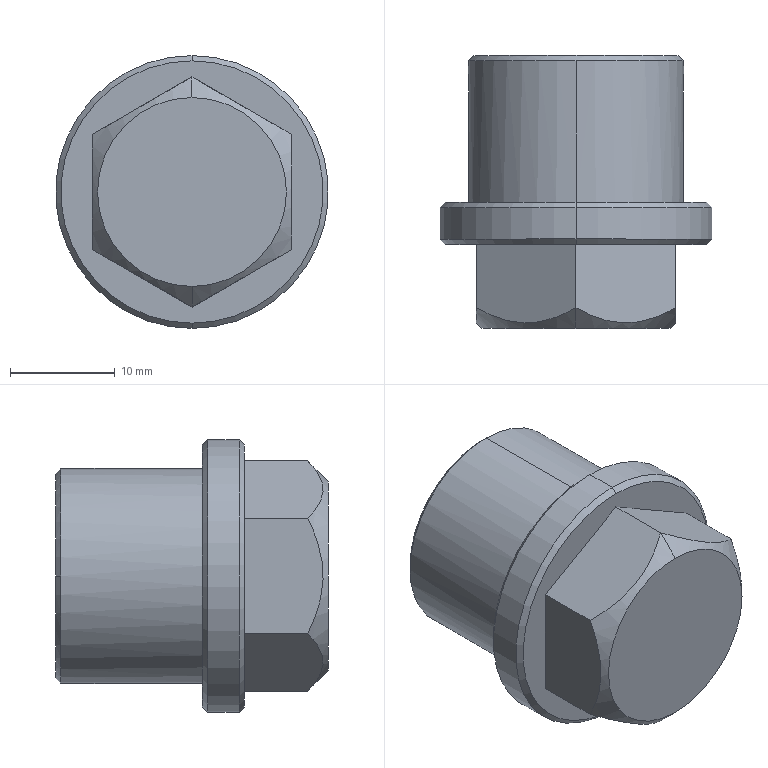Part | STEP file | VD-151208000366A_DN15_X2_76F490 | 1 solid | 22 faces | box 26 x 26 x 26 mm | volume 9182 mm3 | plane 10 | cone 8 | cylinder 4 | commonest cylinder face diameters 20.5 x2 26 x2
STEP:
#1=CARTESIAN_POINT('',(9.75,26.,0.));
#2=VERTEX_POINT('',#1);
#3=CARTESIAN_POINT('',(-9.75,26.,0.));
#4=VERTEX_POINT('',#3);
#5=CARTESIAN_POINT('',(0.,26.,0.));
#6=DIRECTION('',(0.,1.,0.));
#7=DIRECTION('',(1.,0.,0.));
#8=AXIS2_PLACEMENT_3D('',#5,#6,#7);
#9=CIRCLE('',#8,9.75);
#10=EDGE_CURVE('',#2,#4,#9,.T.);
#11=ORIENTED_EDGE('',*,*,#10,.T.);
#12=CARTESIAN_POINT('',(0.,26.,0.));
#13=DIRECTION('',(0.,1.,0.));
#14=DIRECTION('',(-1.,0.,0.));
#15=AXIS2_PLACEMENT_3D('',#12,#13,#14);
#16=CIRCLE('',#15,9.75);
#17=EDGE_CURVE('',#4,#2,#16,.T.);
#18=ORIENTED_EDGE('',*,*,#17,.T.);
#19=EDGE_LOOP('',(#11,#18));
#20=FACE_OUTER_BOUND('',#19,.T.);
#21=CARTESIAN_POINT('',(0.,26.,0.));
#22=DIRECTION('',(0.,1.,0.));
#23=DIRECTION('',(1.,0.,0.));
#24=AXIS2_PLACEMENT_3D('',#21,#22,#23);
#25=PLANE('',#24);
#26=ADVANCED_FACE('',(#20),#25,.T.);
#27=CARTESIAN_POINT('',(-10.25,25.5,0.));
#28=VERTEX_POINT('',#27);
#29=CARTESIAN_POINT('',(-10.25,25.5,0.));
#30=DIRECTION('',(0.7071,0.7071,0.));
#31=VECTOR('',#30,1000.);
#32=LINE('',#29,#31);
#33=EDGE_CURVE('',#28,#4,#32,.T.);
#34=ORIENTED_EDGE('',*,*,#33,.F.);
#35=CARTESIAN_POINT('',(0.,25.5,10.25));
#36=VERTEX_POINT('',#35);
#37=CARTESIAN_POINT('',(0.,25.5,0.));
#38=DIRECTION('',(0.,1.,0.));
#39=DIRECTION('',(-1.,0.,0.));
#40=AXIS2_PLACEMENT_3D('',#37,#38,#39);
#41=CIRCLE('',#40,10.25);
#42=EDGE_CURVE('',#28,#36,#41,.T.);
#43=ORIENTED_EDGE('',*,*,#42,.T.);
#44=CARTESIAN_POINT('',(10.25,25.5,0.));
#45=VERTEX_POINT('',#44);
#46=CARTESIAN_POINT('',(0.,25.5,0.));
#47=DIRECTION('',(0.,1.,0.));
#48=DIRECTION('',(0.,0.,1.));
#49=AXIS2_PLACEMENT_3D('',#46,#47,#48);
#50=CIRCLE('',#49,10.25);
#51=EDGE_CURVE('',#36,#45,#50,.T.);
#52=ORIENTED_EDGE('',*,*,#51,.T.);
#53=CARTESIAN_POINT('',(10.25,25.5,0.));
#54=DIRECTION('',(-0.7071,0.7071,0.));
#55=VECTOR('',#54,1000.);
#56=LINE('',#53,#55);
#57=EDGE_CURVE('',#45,#2,#56,.T.);
#58=ORIENTED_EDGE('',*,*,#57,.T.);
#59=ORIENTED_EDGE('',*,*,#17,.F.);
#60=EDGE_LOOP('',(#34,#43,#52,#58,#59));
#61=FACE_OUTER_BOUND('',#60,.T.);
#62=CARTESIAN_POINT('',(0.,25.75,0.));
#63=DIRECTION('',(0.,-1.,0.));
#64=DIRECTION('',(1.,0.,0.));
#65=AXIS2_PLACEMENT_3D('',#62,#63,#64);
#66=CONICAL_SURFACE('',#65,10.,0.7854);
#67=ADVANCED_FACE('',(#61),#66,.T.);
#68=ORIENTED_EDGE('',*,*,#10,.F.);
#69=ORIENTED_EDGE('',*,*,#57,.F.);
#70=CARTESIAN_POINT('',(0.,25.5,-10.25));
#71=VERTEX_POINT('',#70);
#72=CARTESIAN_POINT('',(0.,25.5,0.));
#73=DIRECTION('',(0.,1.,0.));
#74=DIRECTION('',(1.,0.,0.));
#75=AXIS2_PLACEMENT_3D('',#72,#73,#74);
#76=CIRCLE('',#75,10.25);
#77=EDGE_CURVE('',#45,#71,#76,.T.);
#78=ORIENTED_EDGE('',*,*,#77,.T.);
#79=CARTESIAN_POINT('',(0.,25.5,0.));
#80=DIRECTION('',(0.,1.,0.));
#81=DIRECTION('',(0.,0.,-1.));
#82=AXIS2_PLACEMENT_3D('',#79,#80,#81);
#83=CIRCLE('',#82,10.25);
#84=EDGE_CURVE('',#71,#28,#83,.T.);
#85=ORIENTED_EDGE('',*,*,#84,.T.);
#86=ORIENTED_EDGE('',*,*,#33,.T.);
#87=EDGE_LOOP('',(#68,#69,#78,#85,#86));
#88=FACE_OUTER_BOUND('',#87,.T.);
#89=CARTESIAN_POINT('',(0.,25.75,0.));
#90=DIRECTION('',(0.,-1.,0.));
#91=DIRECTION('',(1.,0.,0.));
#92=AXIS2_PLACEMENT_3D('',#89,#90,#91);
#93=CONICAL_SURFACE('',#92,10.,0.7854);
#94=ADVANCED_FACE('',(#88),#93,.T.);
#95=CARTESIAN_POINT('',(0.,12.,10.25));
#96=VERTEX_POINT('',#95);
#97=CARTESIAN_POINT('',(0.,12.,-10.25));
#98=VERTEX_POINT('',#97);
#99=CARTESIAN_POINT('',(0.,12.,0.));
#100=DIRECTION('',(0.,-1.,0.));
#101=DIRECTION('',(0.,0.,1.));
#102=AXIS2_PLACEMENT_3D('',#99,#100,#101);
#103=CIRCLE('',#102,10.25);
#104=EDGE_CURVE('',#96,#98,#103,.T.);
#105=ORIENTED_EDGE('',*,*,#104,.F.);
#106=CARTESIAN_POINT('',(0.,25.5,10.25));
#107=DIRECTION('',(0.,-1.,0.));
#108=VECTOR('',#107,1000.);
#109=LINE('',#106,#108);
#110=EDGE_CURVE('',#36,#96,#109,.T.);
#111=ORIENTED_EDGE('',*,*,#110,.F.);
#112=ORIENTED_EDGE('',*,*,#42,.F.);
#113=ORIENTED_EDGE('',*,*,#84,.F.);
#114=CARTESIAN_POINT('',(0.,25.5,-10.25));
#115=DIRECTION('',(0.,-1.,0.));
#116=VECTOR('',#115,1000.);
#117=LINE('',#114,#116);
#118=EDGE_CURVE('',#71,#98,#117,.T.);
#119=ORIENTED_EDGE('',*,*,#118,.T.);
#120=EDGE_LOOP('',(#105,#111,#112,#113,#119));
#121=FACE_OUTER_BOUND('',#120,.T.);
#122=CARTESIAN_POINT('',(0.,26.,0.));
#123=DIRECTION('',(0.,1.,0.));
#124=DIRECTION('',(0.,0.,1.));
#125=AXIS2_PLACEMENT_3D('',#122,#123,#124);
#126=CYLINDRICAL_SURFACE('',#125,10.25);
#127=ADVANCED_FACE('',(#121),#126,.T.);
#128=ORIENTED_EDGE('',*,*,#118,.F.);
#129=ORIENTED_EDGE('',*,*,#77,.F.);
#130=ORIENTED_EDGE('',*,*,#51,.F.);
#131=ORIENTED_EDGE('',*,*,#110,.T.);
#132=CARTESIAN_POINT('',(0.,12.,0.));
#133=DIRECTION('',(0.,-1.,0.));
#134=DIRECTION('',(0.,0.,-1.));
#135=AXIS2_PLACEMENT_3D('',#132,#133,#134);
#136=CIRCLE('',#135,10.25);
#137=EDGE_CURVE('',#98,#96,#136,.T.);
#138=ORIENTED_EDGE('',*,*,#137,.F.);
#139=EDGE_LOOP('',(#128,#129,#130,#131,#138));
#140=FACE_OUTER_BOUND('',#139,.T.);
#141=CARTESIAN_POINT('',(0.,26.,0.));
#142=DIRECTION('',(0.,1.,0.));
#143=DIRECTION('',(0.,0.,1.));
#144=AXIS2_PLACEMENT_3D('',#141,#142,#143);
#145=CYLINDRICAL_SURFACE('',#144,10.25);
#146=ADVANCED_FACE('',(#140),#145,.T.);
#147=ORIENTED_EDGE('',*,*,#104,.T.);
#148=ORIENTED_EDGE('',*,*,#137,.T.);
#149=EDGE_LOOP('',(#147,#148));
#150=FACE_BOUND('',#149,.T.);
#151=CARTESIAN_POINT('',(0.,12.,12.5));
#152=VERTEX_POINT('',#151);
#153=CARTESIAN_POINT('',(0.,12.,-12.5));
#154=VERTEX_POINT('',#153);
#155=CARTESIAN_POINT('',(0.,12.,0.));
#156=DIRECTION('',(0.,1.,0.));
#157=DIRECTION('',(0.,0.,1.));
#158=AXIS2_PLACEMENT_3D('',#155,#156,#157);
#159=CIRCLE('',#158,12.5);
#160=EDGE_CURVE('',#152,#154,#159,.T.);
#161=ORIENTED_EDGE('',*,*,#160,.T.);
#162=CARTESIAN_POINT('',(0.,12.,0.));
#163=DIRECTION('',(0.,1.,0.));
#164=DIRECTION('',(0.,0.,-1.));
#165=AXIS2_PLACEMENT_3D('',#162,#163,#164);
#166=CIRCLE('',#165,12.5);
#167=EDGE_CURVE('',#154,#152,#166,.T.);
#168=ORIENTED_EDGE('',*,*,#167,.T.);
#169=EDGE_LOOP('',(#161,#168));
#170=FACE_OUTER_BOUND('',#169,.T.);
#171=CARTESIAN_POINT('',(0.,12.,0.));
#172=DIRECTION('',(0.,1.,0.));
#173=DIRECTION('',(1.,0.,0.));
#174=AXIS2_PLACEMENT_3D('',#171,#172,#173);
#175=PLANE('',#174);
#176=ADVANCED_FACE('',(#150,#170),#175,.T.);
#177=CARTESIAN_POINT('',(0.,11.5,13.));
#178=VERTEX_POINT('',#177);
#179=CARTESIAN_POINT('',(0.,11.5,13.));
#180=DIRECTION('',(0.,0.7071,-0.7071));
#181=VECTOR('',#180,1000.);
#182=LINE('',#179,#181);
#183=EDGE_CURVE('',#178,#152,#182,.T.);
#184=ORIENTED_EDGE('',*,*,#183,.F.);
#185=CARTESIAN_POINT('',(0.,11.5,-13.));
#186=VERTEX_POINT('',#185);
#187=CARTESIAN_POINT('',(0.,11.5,0.));
#188=DIRECTION('',(0.,1.,0.));
#189=DIRECTION('',(0.,0.,1.));
#190=AXIS2_PLACEMENT_3D('',#187,#188,#189);
#191=CIRCLE('',#190,13.);
#192=EDGE_CURVE('',#178,#186,#191,.T.);
#193=ORIENTED_EDGE('',*,*,#192,.T.);
#194=CARTESIAN_POINT('',(0.,11.5,-13.));
#195=DIRECTION('',(0.,0.7071,0.7071));
#196=VECTOR('',#195,1000.);
#197=LINE('',#194,#196);
#198=EDGE_CURVE('',#186,#154,#197,.T.);
#199=ORIENTED_EDGE('',*,*,#198,.T.);
#200=ORIENTED_EDGE('',*,*,#160,.F.);
#201=EDGE_LOOP('',(#184,#193,#199,#200));
#202=FACE_OUTER_BOUND('',#201,.T.);
#203=CARTESIAN_POINT('',(0.,11.75,0.));
#204=DIRECTION('',(0.,-1.,0.));
#205=DIRECTION('',(0.,0.,-1.));
#206=AXIS2_PLACEMENT_3D('',#203,#204,#205);
#207=CONICAL_SURFACE('',#206,12.75,0.7854);
#208=ADVANCED_FACE('',(#202),#207,.T.);
#209=ORIENTED_EDGE('',*,*,#167,.F.);
#210=ORIENTED_EDGE('',*,*,#198,.F.);
#211=CARTESIAN_POINT('',(0.,11.5,0.));
#212=DIRECTION('',(0.,1.,0.));
#213=DIRECTION('',(0.,0.,-1.));
#214=AXIS2_PLACEMENT_3D('',#211,#212,#213);
#215=CIRCLE('',#214,13.);
#216=EDGE_CURVE('',#186,#178,#215,.T.);
#217=ORIENTED_EDGE('',*,*,#216,.T.);
#218=ORIENTED_EDGE('',*,*,#183,.T.);
#219=EDGE_LOOP('',(#209,#210,#217,#218));
#220=FACE_OUTER_BOUND('',#219,.T.);
#221=CARTESIAN_POINT('',(0.,11.75,0.));
#222=DIRECTION('',(0.,-1.,0.));
#223=DIRECTION('',(0.,0.,-1.));
#224=AXIS2_PLACEMENT_3D('',#221,#222,#223);
#225=CONICAL_SURFACE('',#224,12.75,0.7854);
#226=ADVANCED_FACE('',(#220),#225,.T.);
#227=CARTESIAN_POINT('',(0.,8.5,13.));
#228=VERTEX_POINT('',#227);
#229=CARTESIAN_POINT('',(0.,8.5,-13.));
#230=VERTEX_POINT('',#229);
#231=CARTESIAN_POINT('',(0.,8.5,0.));
#232=DIRECTION('',(0.,-1.,0.));
#233=DIRECTION('',(0.,0.,1.));
#234=AXIS2_PLACEMENT_3D('',#231,#232,#233);
#235=CIRCLE('',#234,13.);
#236=EDGE_CURVE('',#228,#230,#235,.T.);
#237=ORIENTED_EDGE('',*,*,#236,.F.);
#238=CARTESIAN_POINT('',(0.,11.5,13.));
#239=DIRECTION('',(0.,-1.,0.));
#240=VECTOR('',#239,1000.);
#241=LINE('',#238,#240);
#242=EDGE_CURVE('',#178,#228,#241,.T.);
#243=ORIENTED_EDGE('',*,*,#242,.F.);
#244=ORIENTED_EDGE('',*,*,#216,.F.);
#245=CARTESIAN_POINT('',(0.,11.5,-13.));
#246=DIRECTION('',(0.,-1.,0.));
#247=VECTOR('',#246,1000.);
#248=LINE('',#245,#247);
#249=EDGE_CURVE('',#186,#230,#248,.T.);
#250=ORIENTED_EDGE('',*,*,#249,.T.);
#251=EDGE_LOOP('',(#237,#243,#244,#250));
#252=FACE_OUTER_BOUND('',#251,.T.);
#253=CARTESIAN_POINT('',(0.,0.,0.));
#254=DIRECTION('',(0.,1.,0.));
#255=DIRECTION('',(0.,0.,1.));
#256=AXIS2_PLACEMENT_3D('',#253,#254,#255);
#257=CYLINDRICAL_SURFACE('',#256,13.);
#258=ADVANCED_FACE('',(#252),#257,.T.);
#259=ORIENTED_EDGE('',*,*,#249,.F.);
#260=ORIENTED_EDGE('',*,*,#192,.F.);
#261=ORIENTED_EDGE('',*,*,#242,.T.);
#262=CARTESIAN_POINT('',(0.,8.5,0.));
#263=DIRECTION('',(0.,-1.,0.));
#264=DIRECTION('',(0.,0.,-1.));
#265=AXIS2_PLACEMENT_3D('',#262,#263,#264);
#266=CIRCLE('',#265,13.);
#267=EDGE_CURVE('',#230,#228,#266,.T.);
#268=ORIENTED_EDGE('',*,*,#267,.F.);
#269=EDGE_LOOP('',(#259,#260,#261,#268));
#270=FACE_OUTER_BOUND('',#269,.T.);
#271=CARTESIAN_POINT('',(0.,0.,0.));
#272=DIRECTION('',(0.,1.,0.));
#273=DIRECTION('',(0.,0.,1.));
#274=AXIS2_PLACEMENT_3D('',#271,#272,#273);
#275=CYLINDRICAL_SURFACE('',#274,13.);
#276=ADVANCED_FACE('',(#270),#275,.T.);
#277=CARTESIAN_POINT('',(0.,0.,9.));
#278=VERTEX_POINT('',#277);
#279=CARTESIAN_POINT('',(0.,0.,-9.));
#280=VERTEX_POINT('',#279);
#281=CARTESIAN_POINT('',(0.,0.,0.));
#282=DIRECTION('',(0.,-1.,0.));
#283=DIRECTION('',(0.,0.,1.));
#284=AXIS2_PLACEMENT_3D('',#281,#282,#283);
#285=CIRCLE('',#284,9.);
#286=EDGE_CURVE('',#278,#280,#285,.T.);
#287=ORIENTED_EDGE('',*,*,#286,.T.);
#288=CARTESIAN_POINT('',(0.,0.,0.));
#289=DIRECTION('',(0.,-1.,0.));
#290=DIRECTION('',(0.,0.,-1.));
#291=AXIS2_PLACEMENT_3D('',#288,#289,#290);
#292=CIRCLE('',#291,9.);
#293=EDGE_CURVE('',#280,#278,#292,.T.);
#294=ORIENTED_EDGE('',*,*,#293,.T.);
#295=EDGE_LOOP('',(#287,#294));
#296=FACE_OUTER_BOUND('',#295,.T.);
#297=CARTESIAN_POINT('',(0.,0.,0.));
#298=DIRECTION('',(0.,1.,0.));
#299=DIRECTION('',(1.,0.,0.));
#300=AXIS2_PLACEMENT_3D('',#297,#298,#299);
#301=PLANE('',#300);
#302=ADVANCED_FACE('',(#296),#301,.F.);
#303=CARTESIAN_POINT('',(0.,1.97,-10.97));
#304=VERTEX_POINT('',#303);
#305=CARTESIAN_POINT('',(0.,1.97,-10.97));
#306=DIRECTION('',(0.,-0.7071,0.7071));
#307=VECTOR('',#306,1000.);
#308=LINE('',#305,#307);
#309=EDGE_CURVE('',#304,#280,#308,.T.);
#310=ORIENTED_EDGE('',*,*,#309,.F.);
#311=CARTESIAN_POINT('',(9.5,1.97,-5.485));
#312=VERTEX_POINT('',#311);
#313=CARTESIAN_POINT('',(0.,1.97,-10.97));
#314=CARTESIAN_POINT('',(0.3939,1.742,-10.742));
#315=CARTESIAN_POINT('',(0.777,1.542,-10.521));
#316=CARTESIAN_POINT('',(1.36,1.273,-10.184));
#317=CARTESIAN_POINT('',(1.552,1.19,-10.073));
#318=CARTESIAN_POINT('',(1.839,1.076,-9.908));
#319=CARTESIAN_POINT('',(1.982,1.022,-9.825));
#320=CARTESIAN_POINT('',(2.148,0.9634,-9.729));
#321=CARTESIAN_POINT('',(2.231,0.9351,-9.681));
#322=CARTESIAN_POINT('',(2.267,0.9233,-9.661));
#323=CARTESIAN_POINT('',(2.29,0.9154,-9.647));
#324=CARTESIAN_POINT('',(2.301,0.9119,-9.641));
#325=CARTESIAN_POINT('',(2.522,0.8396,-9.514));
#326=CARTESIAN_POINT('',(2.728,0.7801,-9.395));
#327=CARTESIAN_POINT('',(3.034,0.7038,-9.218));
#328=CARTESIAN_POINT('',(3.186,0.6688,-9.13));
#329=CARTESIAN_POINT('',(3.364,0.6336,-9.028));
#330=CARTESIAN_POINT('',(3.439,0.6197,-8.984));
#331=CARTESIAN_POINT('',(3.49,0.6107,-8.955));
#332=CARTESIAN_POINT('',(3.514,0.6066,-8.941));
#333=CARTESIAN_POINT('',(3.753,0.5665,-8.803));
#334=CARTESIAN_POINT('',(3.964,0.5403,-8.681));
#335=CARTESIAN_POINT('',(4.279,0.5148,-8.499));
#336=CARTESIAN_POINT('',(4.384,0.5086,-8.438));
#337=CARTESIAN_POINT('',(4.542,0.5028,-8.347));
#338=CARTESIAN_POINT('',(4.594,0.5015,-8.317));
#339=CARTESIAN_POINT('',(4.699,0.5,-8.256));
#340=CARTESIAN_POINT('',(4.753,0.4998,-8.225));
#341=CARTESIAN_POINT('',(5.01,0.5018,-8.077));
#342=CARTESIAN_POINT('',(5.216,0.5123,-7.958));
#343=CARTESIAN_POINT('',(5.525,0.5414,-7.78));
#344=CARTESIAN_POINT('',(5.679,0.5593,-7.691));
#345=CARTESIAN_POINT('',(5.861,0.586,-7.586));
#346=CARTESIAN_POINT('',(5.939,0.5987,-7.541));
#347=CARTESIAN_POINT('',(5.991,0.6074,-7.511));
#348=CARTESIAN_POINT('',(6.018,0.6122,-7.495));
#349=CARTESIAN_POINT('',(6.241,0.652,-7.367));
#350=CARTESIAN_POINT('',(6.439,0.6956,-7.252));
#351=CARTESIAN_POINT('',(6.739,0.7732,-7.079));
#352=CARTESIAN_POINT('',(6.89,0.8151,-6.992));
#353=CARTESIAN_POINT('',(7.067,0.8693,-6.89));
#354=CARTESIAN_POINT('',(7.156,0.8977,-6.838));
#355=CARTESIAN_POINT('',(7.194,0.9102,-6.816));
#356=CARTESIAN_POINT('',(7.219,0.9186,-6.802));
#357=CARTESIAN_POINT('',(7.233,0.9232,-6.794));
#358=CARTESIAN_POINT('',(7.612,1.05,-6.575));
#359=CARTESIAN_POINT('',(7.982,1.199,-6.361));
#360=CARTESIAN_POINT('',(8.737,1.549,-5.925));
#361=CARTESIAN_POINT('',(9.113,1.746,-5.708));
#362=CARTESIAN_POINT('',(9.5,1.97,-5.485));
#363=B_SPLINE_CURVE_WITH_KNOTS('',3,(#313,#314,#315,#316,#317,#318,#319,#320,#321,#322,#323,#324,#325,#326,#327,#328,#329,#330,#331,#332,#333,#334,#335,#336,#337,#338,#339,#340,#341,#342,#343,#344,#345,#346,#347,#348,#349,#350,#351,#352,#353,#354,#355,#356,#357,#358,#359,#360,#361,#362),.UNSPECIFIED.,.F.,.F.,(4,2,2,1,1,1,2,2,2,1,1,2,2,2,2,2,2,2,1,1,2,2,2,1,1,1,2,2,2,4),(0.,0.125,0.1875,0.2188,0.2344,0.2422,0.2461,0.25,0.3125,0.3438,0.3594,0.3672,0.375,0.4375,0.4688,0.4844,0.5,0.5625,0.5938,0.6094,0.6172,0.625,0.6875,0.7188,0.7344,0.7422,0.7461,0.75,0.875,1.),.UNSPECIFIED.);
#364=EDGE_CURVE('',#304,#312,#363,.T.);
#365=ORIENTED_EDGE('',*,*,#364,.T.);
#366=CARTESIAN_POINT('',(9.5,1.97,5.485));
#367=VERTEX_POINT('',#366);
#368=CARTESIAN_POINT('',(9.5,1.97,-5.485));
#369=CARTESIAN_POINT('',(9.5,1.742,-5.03));
#370=CARTESIAN_POINT('',(9.5,1.542,-4.588));
#371=CARTESIAN_POINT('',(9.5,1.273,-3.915));
#372=CARTESIAN_POINT('',(9.5,1.19,-3.693));
#373=CARTESIAN_POINT('',(9.5,1.076,-3.361));
#374=CARTESIAN_POINT('',(9.5,1.022,-3.196));
#375=CARTESIAN_POINT('',(9.5,0.9634,-3.004));
#376=CARTESIAN_POINT('',(9.5,0.9351,-2.908));
#377=CARTESIAN_POINT('',(9.5,0.9233,-2.867));
#378=CARTESIAN_POINT('',(9.5,0.9154,-2.84));
#379=CARTESIAN_POINT('',(9.5,0.9119,-2.828));
#380=CARTESIAN_POINT('',(9.5,0.8396,-2.573));
#381=CARTESIAN_POINT('',(9.5,0.7801,-2.335));
#382=CARTESIAN_POINT('',(9.5,0.7038,-1.982));
#383=CARTESIAN_POINT('',(9.5,0.6688,-1.806));
#384=CARTESIAN_POINT('',(9.5,0.6336,-1.601));
#385=CARTESIAN_POINT('',(9.5,0.6197,-1.513));
#386=CARTESIAN_POINT('',(9.5,0.6107,-1.455));
#387=CARTESIAN_POINT('',(9.5,0.6066,-1.427));
#388=CARTESIAN_POINT('',(9.5,0.5665,-1.151));
#389=CARTESIAN_POINT('',(9.5,0.5403,-0.9076));
#390=CARTESIAN_POINT('',(9.5,0.5148,-0.5434));
#391=CARTESIAN_POINT('',(9.5,0.5086,-0.4221));
#392=CARTESIAN_POINT('',(9.5,0.5028,-0.2403));
#393=CARTESIAN_POINT('',(9.5,0.5015,-0.1796));
#394=CARTESIAN_POINT('',(9.5,0.5,-0.05831));
#395=CARTESIAN_POINT('',(9.5,0.4998,0.003679));
#396=CARTESIAN_POINT('',(9.5,0.5018,0.3007));
#397=CARTESIAN_POINT('',(9.5,0.5123,0.5378));
#398=CARTESIAN_POINT('',(9.5,0.5414,0.8945));
#399=CARTESIAN_POINT('',(9.5,0.5533,1.014));
#400=CARTESIAN_POINT('',(9.5,0.5745,1.193));
#401=CARTESIAN_POINT('',(9.5,0.586,1.282));
#402=CARTESIAN_POINT('',(9.5,0.5987,1.372));
#403=CARTESIAN_POINT('',(9.5,0.6074,1.432));
#404=CARTESIAN_POINT('',(9.5,0.6122,1.464));
#405=CARTESIAN_POINT('',(9.5,0.652,1.721));
#406=CARTESIAN_POINT('',(9.5,0.6956,1.951));
#407=CARTESIAN_POINT('',(9.5,0.7732,2.297));
#408=CARTESIAN_POINT('',(9.5,0.8151,2.471));
#409=CARTESIAN_POINT('',(9.5,0.8693,2.675));
#410=CARTESIAN_POINT('',(9.5,0.8977,2.778));
#411=CARTESIAN_POINT('',(9.5,0.9102,2.822));
#412=CARTESIAN_POINT('',(9.5,0.9186,2.851));
#413=CARTESIAN_POINT('',(9.5,0.9232,2.867));
#414=CARTESIAN_POINT('',(9.5,1.05,3.304));
#415=CARTESIAN_POINT('',(9.5,1.199,3.732));
#416=CARTESIAN_POINT('',(9.5,1.549,4.604));
#417=CARTESIAN_POINT('',(9.5,1.746,5.038));
#418=CARTESIAN_POINT('',(9.5,1.97,5.485));
#419=B_SPLINE_CURVE_WITH_KNOTS('',3,(#368,#369,#370,#371,#372,#373,#374,#375,#376,#377,#378,#379,#380,#381,#382,#383,#384,#385,#386,#387,#388,#389,#390,#391,#392,#393,#394,#395,#396,#397,#398,#399,#400,#401,#402,#403,#404,#405,#406,#407,#408,#409,#410,#411,#412,#413,#414,#415,#416,#417,#418),.UNSPECIFIED.,.F.,.F.,(4,2,2,1,1,1,2,2,2,1,1,2,2,2,2,2,2,2,2,1,2,2,2,1,1,1,2,2,2,4),(0.,0.125,0.1875,0.2188,0.2344,0.2422,0.2461,0.25,0.3125,0.3438,0.3594,0.3672,0.375,0.4375,0.4688,0.4844,0.5,0.5625,0.5938,0.6094,0.6172,0.625,0.6875,0.7188,0.7344,0.7422,0.7461,0.75,0.875,1.),.UNSPECIFIED.);
#420=EDGE_CURVE('',#312,#367,#419,.T.);
#421=ORIENTED_EDGE('',*,*,#420,.T.);
#422=CARTESIAN_POINT('',(0.,1.97,10.97));
#423=VERTEX_POINT('',#422);
#424=CARTESIAN_POINT('',(9.5,1.97,5.485));
#425=CARTESIAN_POINT('',(9.106,1.742,5.712));
#426=CARTESIAN_POINT('',(8.723,1.542,5.933));
#427=CARTESIAN_POINT('',(8.14,1.273,6.27));
#428=CARTESIAN_POINT('',(7.948,1.19,6.381));
#429=CARTESIAN_POINT('',(7.661,1.076,6.546));
#430=CARTESIAN_POINT('',(7.518,1.022,6.629));
#431=CARTESIAN_POINT('',(7.352,0.9634,6.725));
#432=CARTESIAN_POINT('',(7.269,0.9351,6.773));
#433=CARTESIAN_POINT('',(7.233,0.9233,6.793));
#434=CARTESIAN_POINT('',(7.21,0.9154,6.807));
#435=CARTESIAN_POINT('',(7.199,0.9119,6.813));
#436=CARTESIAN_POINT('',(6.978,0.8396,6.941));
#437=CARTESIAN_POINT('',(6.772,0.7801,7.06));
#438=CARTESIAN_POINT('',(6.466,0.7038,7.236));
#439=CARTESIAN_POINT('',(6.314,0.6688,7.324));
#440=CARTESIAN_POINT('',(6.136,0.6336,7.427));
#441=CARTESIAN_POINT('',(6.061,0.6197,7.471));
#442=CARTESIAN_POINT('',(6.01,0.6107,7.5));
#443=CARTESIAN_POINT('',(5.986,0.6066,7.514));
#444=CARTESIAN_POINT('',(5.747,0.5665,7.652));
#445=CARTESIAN_POINT('',(5.536,0.5403,7.774));
#446=CARTESIAN_POINT('',(5.221,0.5148,7.956));
#447=CARTESIAN_POINT('',(5.116,0.5086,8.016));
#448=CARTESIAN_POINT('',(4.958,0.5028,8.107));
#449=CARTESIAN_POINT('',(4.906,0.5015,8.137));
#450=CARTESIAN_POINT('',(4.801,0.5,8.198));
#451=CARTESIAN_POINT('',(4.747,0.4998,8.229));
#452=CARTESIAN_POINT('',(4.49,0.5018,8.378));
#453=CARTESIAN_POINT('',(4.284,0.5123,8.496));
#454=CARTESIAN_POINT('',(3.975,0.5414,8.675));
#455=CARTESIAN_POINT('',(3.872,0.5533,8.734));
#456=CARTESIAN_POINT('',(3.717,0.5745,8.824));
#457=CARTESIAN_POINT('',(3.639,0.586,8.869));
#458=CARTESIAN_POINT('',(3.562,0.5987,8.914));
#459=CARTESIAN_POINT('',(3.51,0.6074,8.944));
#460=CARTESIAN_POINT('',(3.482,0.6122,8.959));
#461=CARTESIAN_POINT('',(3.259,0.652,9.088));
#462=CARTESIAN_POINT('',(3.061,0.6956,9.203));
#463=CARTESIAN_POINT('',(2.761,0.7732,9.376));
#464=CARTESIAN_POINT('',(2.61,0.8151,9.463));
#465=CARTESIAN_POINT('',(2.433,0.8693,9.565));
#466=CARTESIAN_POINT('',(2.345,0.8977,9.616));
#467=CARTESIAN_POINT('',(2.306,0.9102,9.638));
#468=CARTESIAN_POINT('',(2.281,0.9186,9.653));
#469=CARTESIAN_POINT('',(2.267,0.9232,9.661));
#470=CARTESIAN_POINT('',(1.888,1.05,9.879));
#471=CARTESIAN_POINT('',(1.518,1.199,10.093));
#472=CARTESIAN_POINT('',(0.763,1.549,10.529));
#473=CARTESIAN_POINT('',(0.3866,1.746,10.746));
#474=CARTESIAN_POINT('',(0.,1.97,10.97));
#475=B_SPLINE_CURVE_WITH_KNOTS('',3,(#424,#425,#426,#427,#428,#429,#430,#431,#432,#433,#434,#435,#436,#437,#438,#439,#440,#441,#442,#443,#444,#445,#446,#447,#448,#449,#450,#451,#452,#453,#454,#455,#456,#457,#458,#459,#460,#461,#462,#463,#464,#465,#466,#467,#468,#469,#470,#471,#472,#473,#474),.UNSPECIFIED.,.F.,.F.,(4,2,2,1,1,1,2,2,2,1,1,2,2,2,2,2,2,2,2,1,2,2,2,1,1,1,2,2,2,4),(0.,0.125,0.1875,0.2187,0.2344,0.2422,0.2461,0.25,0.3125,0.3437,0.3594,0.3672,0.375,0.4375,0.4688,0.4844,0.5,0.5625,0.5938,0.6094,0.6172,0.625,0.6875,0.7188,0.7344,0.7422,0.7461,0.75,0.875,1.),.UNSPECIFIED.);
#476=EDGE_CURVE('',#367,#423,#475,.T.);
#477=ORIENTED_EDGE('',*,*,#476,.T.);
#478=CARTESIAN_POINT('',(0.,1.97,10.97));
#479=DIRECTION('',(0.,-0.7071,-0.7071));
#480=VECTOR('',#479,1000.);
#481=LINE('',#478,#480);
#482=EDGE_CURVE('',#423,#278,#481,.T.);
#483=ORIENTED_EDGE('',*,*,#482,.T.);
#484=ORIENTED_EDGE('',*,*,#293,.F.);
#485=EDGE_LOOP('',(#310,#365,#421,#477,#483,#484));
#486=FACE_OUTER_BOUND('',#485,.T.);
#487=CARTESIAN_POINT('',(0.,0.9848,0.));
#488=DIRECTION('',(0.,1.,0.));
#489=DIRECTION('',(0.,0.,1.));
#490=AXIS2_PLACEMENT_3D('',#487,#488,#489);
#491=CONICAL_SURFACE('',#490,9.985,0.7854);
#492=ADVANCED_FACE('',(#486),#491,.T.);
#493=ORIENTED_EDGE('',*,*,#286,.F.);
#494=ORIENTED_EDGE('',*,*,#482,.F.);
#495=CARTESIAN_POINT('',(-9.5,1.97,5.485));
#496=VERTEX_POINT('',#495);
#497=CARTESIAN_POINT('',(0.,1.97,10.97));
#498=CARTESIAN_POINT('',(-0.3939,1.742,10.742));
#499=CARTESIAN_POINT('',(-0.777,1.542,10.521));
#500=CARTESIAN_POINT('',(-1.36,1.273,10.184));
#501=CARTESIAN_POINT('',(-1.552,1.19,10.073));
#502=CARTESIAN_POINT('',(-1.839,1.076,9.908));
#503=CARTESIAN_POINT('',(-1.982,1.022,9.825));
#504=CARTESIAN_POINT('',(-2.148,0.9634,9.729));
#505=CARTESIAN_POINT('',(-2.231,0.9351,9.681));
#506=CARTESIAN_POINT('',(-2.267,0.9233,9.661));
#507=CARTESIAN_POINT('',(-2.29,0.9154,9.647));
#508=CARTESIAN_POINT('',(-2.301,0.9119,9.641));
#509=CARTESIAN_POINT('',(-2.522,0.8396,9.514));
#510=CARTESIAN_POINT('',(-2.728,0.7801,9.395));
#511=CARTESIAN_POINT('',(-3.034,0.7038,9.218));
#512=CARTESIAN_POINT('',(-3.186,0.6688,9.13));
#513=CARTESIAN_POINT('',(-3.364,0.6336,9.028));
#514=CARTESIAN_POINT('',(-3.439,0.6197,8.984));
#515=CARTESIAN_POINT('',(-3.49,0.6107,8.955));
#516=CARTESIAN_POINT('',(-3.514,0.6066,8.941));
#517=CARTESIAN_POINT('',(-3.753,0.5665,8.803));
#518=CARTESIAN_POINT('',(-3.964,0.5403,8.681));
#519=CARTESIAN_POINT('',(-4.279,0.5148,8.499));
#520=CARTESIAN_POINT('',(-4.384,0.5086,8.438));
#521=CARTESIAN_POINT('',(-4.542,0.5028,8.347));
#522=CARTESIAN_POINT('',(-4.594,0.5015,8.317));
#523=CARTESIAN_POINT('',(-4.699,0.5,8.256));
#524=CARTESIAN_POINT('',(-4.753,0.4998,8.225));
#525=CARTESIAN_POINT('',(-5.01,0.5018,8.077));
#526=CARTESIAN_POINT('',(-5.216,0.5123,7.958));
#527=CARTESIAN_POINT('',(-5.525,0.5414,7.78));
#528=CARTESIAN_POINT('',(-5.679,0.5593,7.691));
#529=CARTESIAN_POINT('',(-5.861,0.586,7.586));
#530=CARTESIAN_POINT('',(-5.939,0.5987,7.541));
#531=CARTESIAN_POINT('',(-5.991,0.6074,7.511));
#532=CARTESIAN_POINT('',(-6.018,0.6122,7.495));
#533=CARTESIAN_POINT('',(-6.241,0.652,7.367));
#534=CARTESIAN_POINT('',(-6.439,0.6956,7.252));
#535=CARTESIAN_POINT('',(-6.739,0.7732,7.079));
#536=CARTESIAN_POINT('',(-6.89,0.8151,6.992));
#537=CARTESIAN_POINT('',(-7.067,0.8693,6.89));
#538=CARTESIAN_POINT('',(-7.156,0.8977,6.838));
#539=CARTESIAN_POINT('',(-7.194,0.9102,6.816));
#540=CARTESIAN_POINT('',(-7.219,0.9186,6.802));
#541=CARTESIAN_POINT('',(-7.233,0.9232,6.794));
#542=CARTESIAN_POINT('',(-7.612,1.05,6.575));
#543=CARTESIAN_POINT('',(-7.982,1.199,6.361));
#544=CARTESIAN_POINT('',(-8.737,1.549,5.925));
#545=CARTESIAN_POINT('',(-9.113,1.746,5.708));
#546=CARTESIAN_POINT('',(-9.5,1.97,5.485));
#547=B_SPLINE_CURVE_WITH_KNOTS('',3,(#497,#498,#499,#500,#501,#502,#503,#504,#505,#506,#507,#508,#509,#510,#511,#512,#513,#514,#515,#516,#517,#518,#519,#520,#521,#522,#523,#524,#525,#526,#527,#528,#529,#530,#531,#532,#533,#534,#535,#536,#537,#538,#539,#540,#541,#542,#543,#544,#545,#546),.UNSPECIFIED.,.F.,.F.,(4,2,2,1,1,1,2,2,2,1,1,2,2,2,2,2,2,2,1,1,2,2,2,1,1,1,2,2,2,4),(0.,0.125,0.1875,0.2188,0.2344,0.2422,0.2461,0.25,0.3125,0.3438,0.3594,0.3672,0.375,0.4375,0.4688,0.4844,0.5,0.5625,0.5938,0.6094,0.6172,0.625,0.6875,0.7188,0.7344,0.7422,0.7461,0.75,0.875,1.),.UNSPECIFIED.);
#548=EDGE_CURVE('',#423,#496,#547,.T.);
#549=ORIENTED_EDGE('',*,*,#548,.T.);
#550=CARTESIAN_POINT('',(-9.5,1.97,-5.485));
#551=VERTEX_POINT('',#550);
#552=CARTESIAN_POINT('',(-9.5,1.97,5.485));
#553=CARTESIAN_POINT('',(-9.5,1.742,5.03));
#554=CARTESIAN_POINT('',(-9.5,1.542,4.588));
#555=CARTESIAN_POINT('',(-9.5,1.273,3.915));
#556=CARTESIAN_POINT('',(-9.5,1.19,3.693));
#557=CARTESIAN_POINT('',(-9.5,1.076,3.361));
#558=CARTESIAN_POINT('',(-9.5,1.022,3.196));
#559=CARTESIAN_POINT('',(-9.5,0.9634,3.004));
#560=CARTESIAN_POINT('',(-9.5,0.9351,2.908));
#561=CARTESIAN_POINT('',(-9.5,0.9233,2.867));
#562=CARTESIAN_POINT('',(-9.5,0.9154,2.84));
#563=CARTESIAN_POINT('',(-9.5,0.9119,2.828));
#564=CARTESIAN_POINT('',(-9.5,0.8396,2.573));
#565=CARTESIAN_POINT('',(-9.5,0.7801,2.335));
#566=CARTESIAN_POINT('',(-9.5,0.7038,1.982));
#567=CARTESIAN_POINT('',(-9.5,0.6688,1.806));
#568=CARTESIAN_POINT('',(-9.5,0.6336,1.601));
#569=CARTESIAN_POINT('',(-9.5,0.6197,1.513));
#570=CARTESIAN_POINT('',(-9.5,0.6107,1.455));
#571=CARTESIAN_POINT('',(-9.5,0.6066,1.427));
#572=CARTESIAN_POINT('',(-9.5,0.5665,1.151));
#573=CARTESIAN_POINT('',(-9.5,0.5403,0.9076));
#574=CARTESIAN_POINT('',(-9.5,0.5148,0.5434));
#575=CARTESIAN_POINT('',(-9.5,0.5086,0.4221));
#576=CARTESIAN_POINT('',(-9.5,0.5028,0.2403));
#577=CARTESIAN_POINT('',(-9.5,0.5015,0.1796));
#578=CARTESIAN_POINT('',(-9.5,0.5,0.05831));
#579=CARTESIAN_POINT('',(-9.5,0.4998,-0.003679));
#580=CARTESIAN_POINT('',(-9.5,0.5018,-0.3007));
#581=CARTESIAN_POINT('',(-9.5,0.5123,-0.5378));
#582=CARTESIAN_POINT('',(-9.5,0.5414,-0.8945));
#583=CARTESIAN_POINT('',(-9.5,0.5533,-1.014));
#584=CARTESIAN_POINT('',(-9.5,0.5745,-1.193));
#585=CARTESIAN_POINT('',(-9.5,0.586,-1.282));
#586=CARTESIAN_POINT('',(-9.5,0.5987,-1.372));
#587=CARTESIAN_POINT('',(-9.5,0.6074,-1.432));
#588=CARTESIAN_POINT('',(-9.5,0.6122,-1.464));
#589=CARTESIAN_POINT('',(-9.5,0.652,-1.721));
#590=CARTESIAN_POINT('',(-9.5,0.6956,-1.951));
#591=CARTESIAN_POINT('',(-9.5,0.7732,-2.297));
#592=CARTESIAN_POINT('',(-9.5,0.8151,-2.471));
#593=CARTESIAN_POINT('',(-9.5,0.8693,-2.675));
#594=CARTESIAN_POINT('',(-9.5,0.8977,-2.778));
#595=CARTESIAN_POINT('',(-9.5,0.9102,-2.822));
#596=CARTESIAN_POINT('',(-9.5,0.9186,-2.851));
#597=CARTESIAN_POINT('',(-9.5,0.9232,-2.867));
#598=CARTESIAN_POINT('',(-9.5,1.05,-3.304));
#599=CARTESIAN_POINT('',(-9.5,1.199,-3.732));
#600=CARTESIAN_POINT('',(-9.5,1.549,-4.604));
#601=CARTESIAN_POINT('',(-9.5,1.746,-5.038));
#602=CARTESIAN_POINT('',(-9.5,1.97,-5.485));
#603=B_SPLINE_CURVE_WITH_KNOTS('',3,(#552,#553,#554,#555,#556,#557,#558,#559,#560,#561,#562,#563,#564,#565,#566,#567,#568,#569,#570,#571,#572,#573,#574,#575,#576,#577,#578,#579,#580,#581,#582,#583,#584,#585,#586,#587,#588,#589,#590,#591,#592,#593,#594,#595,#596,#597,#598,#599,#600,#601,#602),.UNSPECIFIED.,.F.,.F.,(4,2,2,1,1,1,2,2,2,1,1,2,2,2,2,2,2,2,2,1,2,2,2,1,1,1,2,2,2,4),(0.,0.125,0.1875,0.2187,0.2344,0.2422,0.2461,0.25,0.3125,0.3437,0.3594,0.3672,0.375,0.4375,0.4687,0.4844,0.5,0.5625,0.5937,0.6094,0.6172,0.625,0.6875,0.7187,0.7344,0.7422,0.7461,0.75,0.875,1.),.UNSPECIFIED.);
#604=EDGE_CURVE('',#496,#551,#603,.T.);
#605=ORIENTED_EDGE('',*,*,#604,.T.);
#606=CARTESIAN_POINT('',(-9.5,1.97,-5.485));
#607=CARTESIAN_POINT('',(-9.106,1.742,-5.712));
#608=CARTESIAN_POINT('',(-8.723,1.542,-5.933));
#609=CARTESIAN_POINT('',(-8.14,1.273,-6.27));
#610=CARTESIAN_POINT('',(-7.948,1.19,-6.381));
#611=CARTESIAN_POINT('',(-7.661,1.076,-6.546));
#612=CARTESIAN_POINT('',(-7.518,1.022,-6.629));
#613=CARTESIAN_POINT('',(-7.352,0.9634,-6.725));
#614=CARTESIAN_POINT('',(-7.269,0.9351,-6.773));
#615=CARTESIAN_POINT('',(-7.233,0.9233,-6.793));
#616=CARTESIAN_POINT('',(-7.21,0.9154,-6.807));
#617=CARTESIAN_POINT('',(-7.199,0.9119,-6.813));
#618=CARTESIAN_POINT('',(-6.978,0.8396,-6.941));
#619=CARTESIAN_POINT('',(-6.772,0.7801,-7.06));
#620=CARTESIAN_POINT('',(-6.466,0.7038,-7.236));
#621=CARTESIAN_POINT('',(-6.314,0.6688,-7.324));
#622=CARTESIAN_POINT('',(-6.136,0.6336,-7.427));
#623=CARTESIAN_POINT('',(-6.061,0.6197,-7.471));
#624=CARTESIAN_POINT('',(-6.01,0.6107,-7.5));
#625=CARTESIAN_POINT('',(-5.986,0.6066,-7.514));
#626=CARTESIAN_POINT('',(-5.747,0.5665,-7.652));
#627=CARTESIAN_POINT('',(-5.536,0.5403,-7.774));
#628=CARTESIAN_POINT('',(-5.221,0.5148,-7.956));
#629=CARTESIAN_POINT('',(-5.116,0.5086,-8.016));
#630=CARTESIAN_POINT('',(-4.958,0.5028,-8.107));
#631=CARTESIAN_POINT('',(-4.906,0.5015,-8.137));
#632=CARTESIAN_POINT('',(-4.801,0.5,-8.198));
#633=CARTESIAN_POINT('',(-4.747,0.4998,-8.229));
#634=CARTESIAN_POINT('',(-4.49,0.5018,-8.378));
#635=CARTESIAN_POINT('',(-4.284,0.5123,-8.496));
#636=CARTESIAN_POINT('',(-3.975,0.5414,-8.675));
#637=CARTESIAN_POINT('',(-3.872,0.5533,-8.734));
#638=CARTESIAN_POINT('',(-3.717,0.5745,-8.824));
#639=CARTESIAN_POINT('',(-3.639,0.586,-8.869));
#640=CARTESIAN_POINT('',(-3.562,0.5987,-8.914));
#641=CARTESIAN_POINT('',(-3.51,0.6074,-8.944));
#642=CARTESIAN_POINT('',(-3.482,0.6122,-8.959));
#643=CARTESIAN_POINT('',(-3.259,0.652,-9.088));
#644=CARTESIAN_POINT('',(-3.061,0.6956,-9.203));
#645=CARTESIAN_POINT('',(-2.761,0.7732,-9.376));
#646=CARTESIAN_POINT('',(-2.61,0.8151,-9.463));
#647=CARTESIAN_POINT('',(-2.433,0.8693,-9.565));
#648=CARTESIAN_POINT('',(-2.345,0.8977,-9.616));
#649=CARTESIAN_POINT('',(-2.306,0.9102,-9.638));
#650=CARTESIAN_POINT('',(-2.281,0.9186,-9.653));
#651=CARTESIAN_POINT('',(-2.267,0.9232,-9.661));
#652=CARTESIAN_POINT('',(-1.888,1.05,-9.879));
#653=CARTESIAN_POINT('',(-1.518,1.199,-10.093));
#654=CARTESIAN_POINT('',(-0.763,1.549,-10.529));
#655=CARTESIAN_POINT('',(-0.3866,1.746,-10.746));
#656=CARTESIAN_POINT('',(0.,1.97,-10.97));
#657=B_SPLINE_CURVE_WITH_KNOTS('',3,(#606,#607,#608,#609,#610,#611,#612,#613,#614,#615,#616,#617,#618,#619,#620,#621,#622,#623,#624,#625,#626,#627,#628,#629,#630,#631,#632,#633,#634,#635,#636,#637,#638,#639,#640,#641,#642,#643,#644,#645,#646,#647,#648,#649,#650,#651,#652,#653,#654,#655,#656),.UNSPECIFIED.,.F.,.F.,(4,2,2,1,1,1,2,2,2,1,1,2,2,2,2,2,2,2,2,1,2,2,2,1,1,1,2,2,2,4),(0.,0.125,0.1875,0.2188,0.2344,0.2422,0.2461,0.25,0.3125,0.3437,0.3594,0.3672,0.375,0.4375,0.4687,0.4844,0.5,0.5625,0.5937,0.6094,0.6172,0.625,0.6875,0.7187,0.7344,0.7422,0.7461,0.75,0.875,1.),.UNSPECIFIED.);
#658=EDGE_CURVE('',#551,#304,#657,.T.);
#659=ORIENTED_EDGE('',*,*,#658,.T.);
#660=ORIENTED_EDGE('',*,*,#309,.T.);
#661=EDGE_LOOP('',(#493,#494,#549,#605,#659,#660));
#662=FACE_OUTER_BOUND('',#661,.T.);
#663=CARTESIAN_POINT('',(0.,0.9848,0.));
#664=DIRECTION('',(0.,1.,0.));
#665=DIRECTION('',(0.,0.,1.));
#666=AXIS2_PLACEMENT_3D('',#663,#664,#665);
#667=CONICAL_SURFACE('',#666,9.985,0.7854);
#668=ADVANCED_FACE('',(#662),#667,.T.);
#669=CARTESIAN_POINT('',(0.,8.,-10.97));
#670=VERTEX_POINT('',#669);
#671=CARTESIAN_POINT('',(0.,8.,-10.97));
#672=DIRECTION('',(0.,-1.,0.));
#673=VECTOR('',#672,1000.);
#674=LINE('',#671,#673);
#675=EDGE_CURVE('',#670,#304,#674,.T.);
#676=ORIENTED_EDGE('',*,*,#675,.T.);
#677=ORIENTED_EDGE('',*,*,#658,.F.);
#678=CARTESIAN_POINT('',(-9.5,8.,-5.485));
#679=VERTEX_POINT('',#678);
#680=CARTESIAN_POINT('',(-9.5,8.,-5.485));
#681=DIRECTION('',(0.,-1.,0.));
#682=VECTOR('',#681,1000.);
#683=LINE('',#680,#682);
#684=EDGE_CURVE('',#679,#551,#683,.T.);
#685=ORIENTED_EDGE('',*,*,#684,.F.);
#686=CARTESIAN_POINT('',(0.,8.,-10.97));
#687=DIRECTION('',(-0.866,0.,0.5));
#688=VECTOR('',#687,1000.);
#689=LINE('',#686,#688);
#690=EDGE_CURVE('',#670,#679,#689,.T.);
#691=ORIENTED_EDGE('',*,*,#690,.F.);
#692=EDGE_LOOP('',(#676,#677,#685,#691));
#693=FACE_OUTER_BOUND('',#692,.T.);
#694=CARTESIAN_POINT('',(0.,0.,-10.97));
#695=DIRECTION('',(0.5,0.,0.866));
#696=DIRECTION('',(0.,-1.,0.));
#697=AXIS2_PLACEMENT_3D('',#694,#695,#696);
#698=PLANE('',#697);
#699=ADVANCED_FACE('',(#693),#698,.F.);
#700=CARTESIAN_POINT('',(9.5,8.,-5.485));
#701=VERTEX_POINT('',#700);
#702=CARTESIAN_POINT('',(9.5,8.,-5.485));
#703=DIRECTION('',(0.,-1.,0.));
#704=VECTOR('',#703,1000.);
#705=LINE('',#702,#704);
#706=EDGE_CURVE('',#701,#312,#705,.T.);
#707=ORIENTED_EDGE('',*,*,#706,.T.);
#708=ORIENTED_EDGE('',*,*,#364,.F.);
#709=ORIENTED_EDGE('',*,*,#675,.F.);
#710=CARTESIAN_POINT('',(9.5,8.,-5.485));
#711=DIRECTION('',(-0.866,0.,-0.5));
#712=VECTOR('',#711,1000.);
#713=LINE('',#710,#712);
#714=EDGE_CURVE('',#701,#670,#713,.T.);
#715=ORIENTED_EDGE('',*,*,#714,.F.);
#716=EDGE_LOOP('',(#707,#708,#709,#715));
#717=FACE_OUTER_BOUND('',#716,.T.);
#718=CARTESIAN_POINT('',(9.5,0.,-5.485));
#719=DIRECTION('',(-0.5,0.,0.866));
#720=DIRECTION('',(0.,1.,0.));
#721=AXIS2_PLACEMENT_3D('',#718,#719,#720);
#722=PLANE('',#721);
#723=ADVANCED_FACE('',(#717),#722,.F.);
#724=CARTESIAN_POINT('',(9.5,8.,5.485));
#725=VERTEX_POINT('',#724);
#726=CARTESIAN_POINT('',(9.5,8.,5.485));
#727=DIRECTION('',(0.,-1.,0.));
#728=VECTOR('',#727,1000.);
#729=LINE('',#726,#728);
#730=EDGE_CURVE('',#725,#367,#729,.T.);
#731=ORIENTED_EDGE('',*,*,#730,.T.);
#732=ORIENTED_EDGE('',*,*,#420,.F.);
#733=ORIENTED_EDGE('',*,*,#706,.F.);
#734=CARTESIAN_POINT('',(9.5,8.,-5.485));
#735=DIRECTION('',(0.,0.,1.));
#736=VECTOR('',#735,1000.);
#737=LINE('',#734,#736);
#738=EDGE_CURVE('',#701,#725,#737,.T.);
#739=ORIENTED_EDGE('',*,*,#738,.T.);
#740=EDGE_LOOP('',(#731,#732,#733,#739));
#741=FACE_OUTER_BOUND('',#740,.T.);
#742=CARTESIAN_POINT('',(9.5,0.,5.485));
#743=DIRECTION('',(-1.,0.,0.));
#744=DIRECTION('',(0.,0.,1.));
#745=AXIS2_PLACEMENT_3D('',#742,#743,#744);
#746=PLANE('',#745);
#747=ADVANCED_FACE('',(#741),#746,.F.);
#748=CARTESIAN_POINT('',(0.,8.,10.97));
#749=VERTEX_POINT('',#748);
#750=CARTESIAN_POINT('',(0.,1.97,10.97));
#751=DIRECTION('',(0.,1.,0.));
#752=VECTOR('',#751,1000.);
#753=LINE('',#750,#752);
#754=EDGE_CURVE('',#423,#749,#753,.T.);
#755=ORIENTED_EDGE('',*,*,#754,.F.);
#756=ORIENTED_EDGE('',*,*,#476,.F.);
#757=ORIENTED_EDGE('',*,*,#730,.F.);
#758=CARTESIAN_POINT('',(0.,8.,10.97));
#759=DIRECTION('',(0.866,0.,-0.5));
#760=VECTOR('',#759,1000.);
#761=LINE('',#758,#760);
#762=EDGE_CURVE('',#749,#725,#761,.T.);
#763=ORIENTED_EDGE('',*,*,#762,.F.);
#764=EDGE_LOOP('',(#755,#756,#757,#763));
#765=FACE_OUTER_BOUND('',#764,.T.);
#766=CARTESIAN_POINT('',(0.,0.,10.97));
#767=DIRECTION('',(-0.5,0.,-0.866));
#768=DIRECTION('',(-0.866,0.,0.5));
#769=AXIS2_PLACEMENT_3D('',#766,#767,#768);
#770=PLANE('',#769);
#771=ADVANCED_FACE('',(#765),#770,.F.);
#772=CARTESIAN_POINT('',(-9.5,8.,5.485));
#773=VERTEX_POINT('',#772);
#774=CARTESIAN_POINT('',(-9.5,8.,5.485));
#775=DIRECTION('',(0.,-1.,0.));
#776=VECTOR('',#775,1000.);
#777=LINE('',#774,#776);
#778=EDGE_CURVE('',#773,#496,#777,.T.);
#779=ORIENTED_EDGE('',*,*,#778,.T.);
#780=ORIENTED_EDGE('',*,*,#548,.F.);
#781=ORIENTED_EDGE('',*,*,#754,.T.);
#782=CARTESIAN_POINT('',(-9.5,8.,5.485));
#783=DIRECTION('',(0.866,0.,0.5));
#784=VECTOR('',#783,1000.);
#785=LINE('',#782,#784);
#786=EDGE_CURVE('',#773,#749,#785,.T.);
#787=ORIENTED_EDGE('',*,*,#786,.F.);
#788=EDGE_LOOP('',(#779,#780,#781,#787));
#789=FACE_OUTER_BOUND('',#788,.T.);
#790=CARTESIAN_POINT('',(-9.5,0.,5.485));
#791=DIRECTION('',(0.5,0.,-0.866));
#792=DIRECTION('',(0.,-1.,0.));
#793=AXIS2_PLACEMENT_3D('',#790,#791,#792);
#794=PLANE('',#793);
#795=ADVANCED_FACE('',(#789),#794,.F.);
#796=ORIENTED_EDGE('',*,*,#684,.T.);
#797=ORIENTED_EDGE('',*,*,#604,.F.);
#798=ORIENTED_EDGE('',*,*,#778,.F.);
#799=CARTESIAN_POINT('',(-9.5,8.,5.485));
#800=DIRECTION('',(0.,0.,-1.));
#801=VECTOR('',#800,1000.);
#802=LINE('',#799,#801);
#803=EDGE_CURVE('',#773,#679,#802,.T.);
#804=ORIENTED_EDGE('',*,*,#803,.T.);
#805=EDGE_LOOP('',(#796,#797,#798,#804));
#806=FACE_OUTER_BOUND('',#805,.T.);
#807=CARTESIAN_POINT('',(-9.5,0.,-5.485));
#808=DIRECTION('',(1.,0.,0.));
#809=DIRECTION('',(0.,1.,0.));
#810=AXIS2_PLACEMENT_3D('',#807,#808,#809);
#811=PLANE('',#810);
#812=ADVANCED_FACE('',(#806),#811,.F.);
#813=ORIENTED_EDGE('',*,*,#786,.T.);
#814=ORIENTED_EDGE('',*,*,#762,.T.);
#815=ORIENTED_EDGE('',*,*,#738,.F.);
#816=ORIENTED_EDGE('',*,*,#714,.T.);
#817=ORIENTED_EDGE('',*,*,#690,.T.);
#818=ORIENTED_EDGE('',*,*,#803,.F.);
#819=EDGE_LOOP('',(#813,#814,#815,#816,#817,#818));
#820=FACE_BOUND('',#819,.T.);
#821=CARTESIAN_POINT('',(0.,8.,12.5));
#822=VERTEX_POINT('',#821);
#823=CARTESIAN_POINT('',(0.,8.,-12.5));
#824=VERTEX_POINT('',#823);
#825=CARTESIAN_POINT('',(0.,8.,0.));
#826=DIRECTION('',(0.,-1.,0.));
#827=DIRECTION('',(0.,0.,1.));
#828=AXIS2_PLACEMENT_3D('',#825,#826,#827);
#829=CIRCLE('',#828,12.5);
#830=EDGE_CURVE('',#822,#824,#829,.T.);
#831=ORIENTED_EDGE('',*,*,#830,.T.);
#832=CARTESIAN_POINT('',(0.,8.,0.));
#833=DIRECTION('',(0.,-1.,0.));
#834=DIRECTION('',(0.,0.,-1.));
#835=AXIS2_PLACEMENT_3D('',#832,#833,#834);
#836=CIRCLE('',#835,12.5);
#837=EDGE_CURVE('',#824,#822,#836,.T.);
#838=ORIENTED_EDGE('',*,*,#837,.T.);
#839=EDGE_LOOP('',(#831,#838));
#840=FACE_OUTER_BOUND('',#839,.T.);
#841=CARTESIAN_POINT('',(0.,8.,0.));
#842=DIRECTION('',(0.,-1.,0.));
#843=DIRECTION('',(0.,0.,-1.));
#844=AXIS2_PLACEMENT_3D('',#841,#842,#843);
#845=PLANE('',#844);
#846=ADVANCED_FACE('',(#820,#840),#845,.T.);
#847=CARTESIAN_POINT('',(0.,8.5,-13.));
#848=DIRECTION('',(0.,-0.7071,0.7071));
#849=VECTOR('',#848,1000.);
#850=LINE('',#847,#849);
#851=EDGE_CURVE('',#230,#824,#850,.T.);
#852=ORIENTED_EDGE('',*,*,#851,.F.);
#853=ORIENTED_EDGE('',*,*,#267,.T.);
#854=CARTESIAN_POINT('',(0.,8.5,13.));
#855=DIRECTION('',(0.,-0.7071,-0.7071));
#856=VECTOR('',#855,1000.);
#857=LINE('',#854,#856);
#858=EDGE_CURVE('',#228,#822,#857,.T.);
#859=ORIENTED_EDGE('',*,*,#858,.T.);
#860=ORIENTED_EDGE('',*,*,#837,.F.);
#861=EDGE_LOOP('',(#852,#853,#859,#860));
#862=FACE_OUTER_BOUND('',#861,.T.);
#863=CARTESIAN_POINT('',(0.,8.25,0.));
#864=DIRECTION('',(0.,1.,0.));
#865=DIRECTION('',(0.,0.,1.));
#866=AXIS2_PLACEMENT_3D('',#863,#864,#865);
#867=CONICAL_SURFACE('',#866,12.75,0.7854);
#868=ADVANCED_FACE('',(#862),#867,.T.);
#869=ORIENTED_EDGE('',*,*,#830,.F.);
#870=ORIENTED_EDGE('',*,*,#858,.F.);
#871=ORIENTED_EDGE('',*,*,#236,.T.);
#872=ORIENTED_EDGE('',*,*,#851,.T.);
#873=EDGE_LOOP('',(#869,#870,#871,#872));
#874=FACE_OUTER_BOUND('',#873,.T.);
#875=CARTESIAN_POINT('',(0.,8.25,0.));
#876=DIRECTION('',(0.,1.,0.));
#877=DIRECTION('',(0.,0.,1.));
#878=AXIS2_PLACEMENT_3D('',#875,#876,#877);
#879=CONICAL_SURFACE('',#878,12.75,0.7854);
#880=ADVANCED_FACE('',(#874),#879,.T.);
#881=CLOSED_SHELL('',(#26,#67,#94,#127,#146,#176,#208,#226,#258,#276,#302,#492,#668,#699,#723,#747,#771,#795,#812,#846,#868,#880));
#882=MANIFOLD_SOLID_BREP('',#881);
#883=CARTESIAN_POINT('',(0.,0.,0.));
#884=DIRECTION('',(0.,0.,1.));
#885=DIRECTION('',(1.,0.,0.));
#886=AXIS2_PLACEMENT_3D('',#883,#884,#885);
#887=(LENGTH_UNIT()NAMED_UNIT(*)SI_UNIT(.MILLI.,.METRE.));
#888=UNCERTAINTY_MEASURE_WITH_UNIT(LENGTH_MEASURE(0.00001),#887,'','');
#889=(NAMED_UNIT(*)PLANE_ANGLE_UNIT()SI_UNIT($,.RADIAN.));
#890=(NAMED_UNIT(*)SI_UNIT($,.STERADIAN.)SOLID_ANGLE_UNIT());
#891=(GEOMETRIC_REPRESENTATION_CONTEXT(3)GLOBAL_UNCERTAINTY_ASSIGNED_CONTEXT((#888))GLOBAL_UNIT_ASSIGNED_CONTEXT((#887,#889,#890))REPRESENTATION_CONTEXT('',''));
#892=ADVANCED_BREP_SHAPE_REPRESENTATION('',(#882,#886),#891);